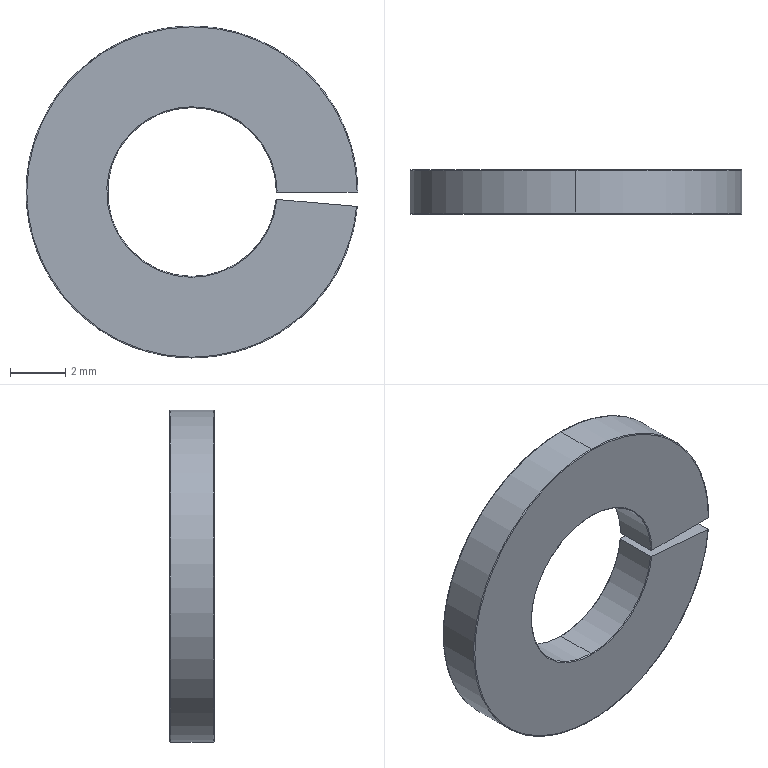Part | SolidWorks | features BaseBody 1 | 1 solid | 22 faces | box 12 x 1.6 x 12 mm | volume 132.312 mm3 | spline 12 | cylinder 6 | plane 4 | commonest cylinder face diameters 6.1 x3 12 x3